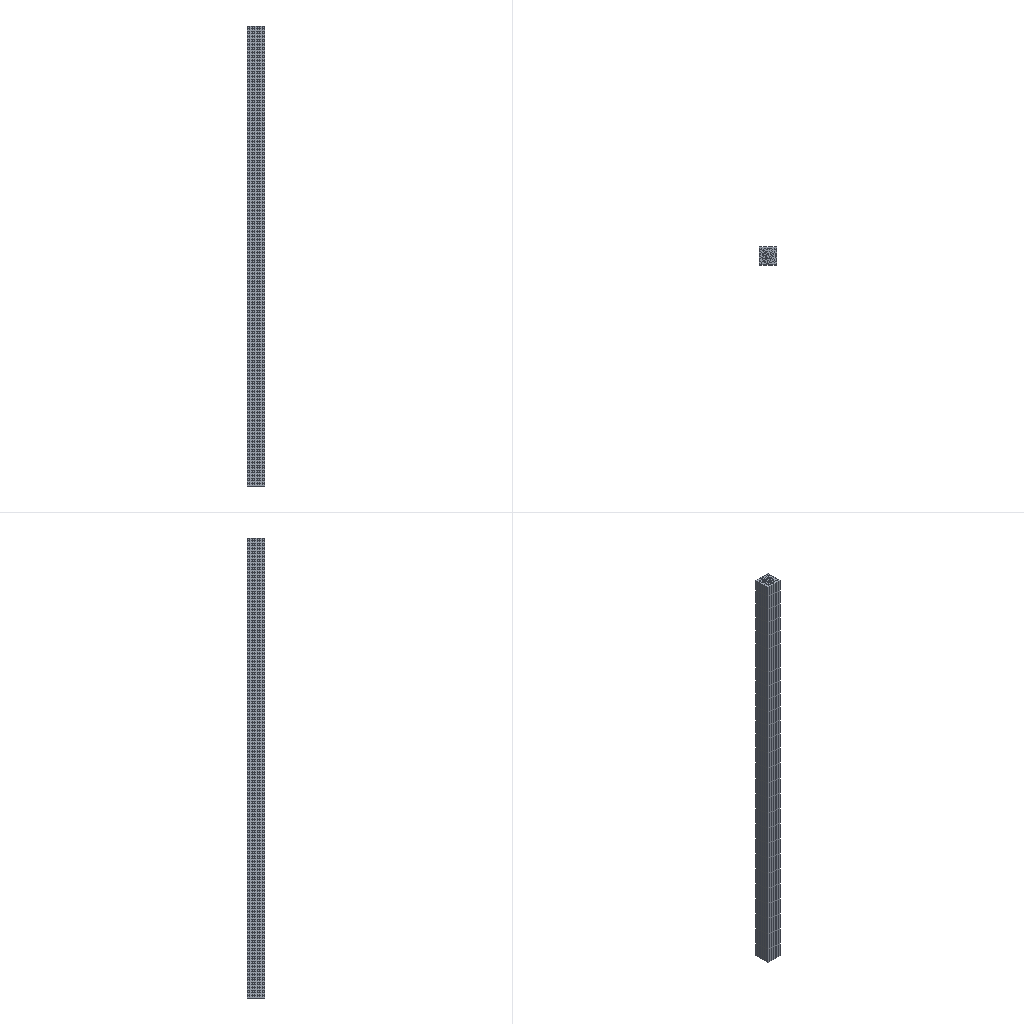Simulation study | abaqus
Set-up summary:
category,name,step,type,value,unit,region
solver,abaqus
solver,version,,,Abaqus/Explicit 2020
units,not stated in the deck,,not stated
analysis,deck,,transient,transient
load_step,Step-1,Step-1,transient,nlgeom=True
contact,interactions,,,general=1 pairs=0 ties=2
load_step,requested,,,1
mesh,nodes,,,18085
mesh,elements,,,14140
element_type,R3D3,,rigid,320
element_type,R3D4,,rigid,2430
element_type,C3D8R,,solid,11390
load,load commands in deck,,count,2
bc,support commands in deck,,count,7
material,MATERIAL-1,,in results
check,setup vs results,,match,"per instance, exact: element labels, types and connectivity; labels of the nodes the elements use; coordinates not compared"
Abaqus input file, long lists of numbers shortened:
*Heading
** Job name: Job-1 Model name: Model-1
** Generated by: Abaqus/CAE 2020
*Preprint, echo=NO, model=NO, history=NO, contact=NO
**
** PARTS
**
*Part, name=Part-1
*Node
      1,  -140.07,   51.876,        4830.
      2,  -140.07,  -148.124,        4830.
** (15494 more lines like these left out)
*Element, type=C3D8R
   1, 1187, 1188, 1184, 1197, 8398, 8399, 8395, 8408
   2, 1188,   70,   69, 1184, 8399, 1423, 1424, 8395
** (11388 more lines like these left out)
*Nset, nset=Set-3, generate
     1,  15496,      1
*Elset, elset=Set-3, generate
     1,  11390,      1
** Section: Section-1
*Solid Section, elset=Set-3, material=Material-1
,
*End Part
**
*Part, name=tool-4
*Node
      1,  -453.731,   383.313,       8282.5
      2,  -453.764,   383.42,   8282.498
** (1486 more lines like these left out)
*Element, type=R3D4
1, 1, 2, 3, 4
2, 5, 6, 7, 8
** (1364 more lines like these left out)
*Element, type=R3D3
516, 234, 184, 627
517, 627, 232, 234
** (250 more lines like these left out)
*Node
   1489,  -468.07,   374.858,    8135.267
*Nset, nset=tool-4-RefPt_, internal
1489,
*Elset, elset=tool-4, generate
    1,  1618,     1
*End Part
**
*Part, name=tool-23
*Node
      1,  -507.527,   342.248,   5134.659
      2,  -434.527,   342.248,   5134.659
** (190 more lines like these left out)
*Element, type=R3D4
 1,   1,   9,  73,  34
 2,   9,  10,  74,  73
** (190 more lines like these left out)
*Node
    193,  -471.027,   342.248,   4234.659
*Nset, nset=tool-23-RefPt_, internal
193,
*Elset, elset=tool-23, generate
   1,  192,    1
*End Part
**
*Part, name=tool-24
*Node
      1,  -464.776,   411.191,    8134.471
      2,  -471.365,     338.524,    8136.062
** (904 more lines like these left out)
*Element, type=R3D3
 1, 366, 270, 325
 2, 328, 258,  54
** (66 more lines like these left out)
*Element, type=R3D4
 24,   1,  18, 273,  64
 25,  58,  59, 278, 320
** (870 more lines like these left out)
*Node
    907,  -471.027,   342.248,   5134.659
*Nset, nset=tool-24-RefPt_, internal
907,
*Elset, elset=tool-24, generate
   1,  940,    1
*End Part
**
**
** ASSEMBLY
**
*Assembly, name=Assembly
**
*Instance, name=tool-4-1, part=tool-4
  427.705,  -213.749,  -6862.641
*End Instance
**
*Instance, name=tool-23-1, part=tool-23
  427.705,  -213.749,  -6862.641
*End Instance
**
*Instance, name=tool-24-1, part=tool-24
  427.705,  -213.749,  -6862.641
*End Instance
**
*Instance, name=Part-1-1, part=Part-1
          0.,   103.752,        5260.
          0.,   103.752,        5260.,           1.,   103.752,        5260.,         180.
*End Instance
**
*Nset, nset=Set-1, instance=Part-1-1
    1,    2,    3,    4,    9,   10,   11,   12,   15,   16,   17,   18,   19,   20,   21,   22
   23,   24,   25,   26,   29,   30,   31,   32,   33,   34,   35,   36,   37,   38,   39,   40
** (306 more lines like these left out)
*Elset, elset=Set-1, instance=Part-1-1
     3,     5,     6,     7,    10,    11,    13,    17,    19,    20,    22,    25,    26,    28,    29,    36
    37,    38,    42,    43,    44,    46,    47,    49,    53,    55,    56,    57,    60,    61,    63,    67
** (261 more lines like these left out)
*Nset, nset=Set-2, instance=tool-23-1
 193,
*Elset, elset=_m_Surf-1_SPOS, internal, instance=tool-23-1, generate
 177,  184,    1
*Surface, type=ELEMENT, name=m_Surf-1
_m_Surf-1_SPOS, SPOS
*Elset, elset=_m_Surf-3_SPOS, internal, instance=tool-24-1, generate
 795,  802,    1
*Surface, type=ELEMENT, name=m_Surf-3
_m_Surf-3_SPOS, SPOS
*Elset, elset=_s_Surf-1_SPOS, internal, instance=tool-24-1, generate
 775,  782,    1
*Surface, type=ELEMENT, name=s_Surf-1
_s_Surf-1_SPOS, SPOS
*Elset, elset=_s_Surf-3_SPOS, internal, instance=tool-4-1, generate
 783,  798,    1
*Surface, type=ELEMENT, name=s_Surf-3
_s_Surf-3_SPOS, SPOS
*Rigid Body, ref node=tool-4-1.tool-4-RefPt_, elset=tool-4-1.tool-4
*Rigid Body, ref node=tool-23-1.tool-23-RefPt_, elset=tool-23-1.tool-23
*Rigid Body, ref node=tool-24-1.tool-24-RefPt_, elset=tool-24-1.tool-24
** Constraint: Constraint-1
*Tie, name=Constraint-1, adjust=yes
s_Surf-1, m_Surf-1
** Constraint: Constraint-2
*Tie, name=Constraint-2, adjust=yes
s_Surf-3, m_Surf-3
*End Assembly
**
** MATERIALS
**
*Material, name=Material-1
*Damage Initiation, criterion=SHEAR
 0.01, 0.8, 0.2
*Damage Evolution, type=DISPLACEMENT
 0.0001,
*Density
 2.2e-09,
*Drucker Prager
34., 0.8, 0.2
*Drucker Prager Hardening
29.,0.
*Elastic
30000., 0.3
**
** INTERACTION PROPERTIES
**
*Surface Interaction, name=IntProp-1
*Friction
 0.3,
*Surface Behavior, pressure-overclosure=HARD
**
** BOUNDARY CONDITIONS
**
** Name: BC-1 Type: 对称/反对称/完全固定
*Boundary
Set-1, ENCASTRE
** ----------------------------------------------------------------
**
** STEP: Step-1
**
*Step, name=Step-1, nlgeom=YES
*Dynamic, Explicit
, 0.3
*Bulk Viscosity
0.06, 1.2
**
** BOUNDARY CONDITIONS
**
** Name: BC-2 Type: 速度/角速度
*Boundary, type=VELOCITY
Set-2, 1, 1
Set-2, 2, 2
Set-2, 3, 3, 10.
Set-2, 4, 4
Set-2, 5, 5
Set-2, 6, 6, 62.8
**
** INTERACTIONS
**
** Interaction: Int-1
*Contact, op=NEW
*Contact Inclusions, ALL EXTERIOR
*Contact Property Assignment
 ,  , IntProp-1
**
** OUTPUT REQUESTS
**
*Restart, write, number interval=1, time marks=NO
**
** FIELD OUTPUT: F-Output-1
**
*Output, field, number interval=50
*Node Output
A, RF, U, V
*Element Output, directions=YES
E, LE, MISES, PE, PEEQ, PEEQVAVG, PEVAVG, S, STATUS, SVAVG
*Contact Output
CFORCE, CSTRESS
**
** HISTORY OUTPUT: H-Output-1
**
*Output, history
*Node Output, nset=Set-2
RF1, RF2, RF3, RM1, RM2, RM3, U1, U2
U3, UR1, UR2, UR3
*End Step
Results summary:
result,step,Step-1,completed,increments=149774 time=0.3/0.3
result,analysis,,,transient
result,last_loadstep,,,1
result,analysis steps,,count,1
result,primary field,,,U
result,reaction total,,FX,-753.379,model units
result,reaction total,,FY,2786.35,model units
result,reaction total,,FZ,-6502.909,model units